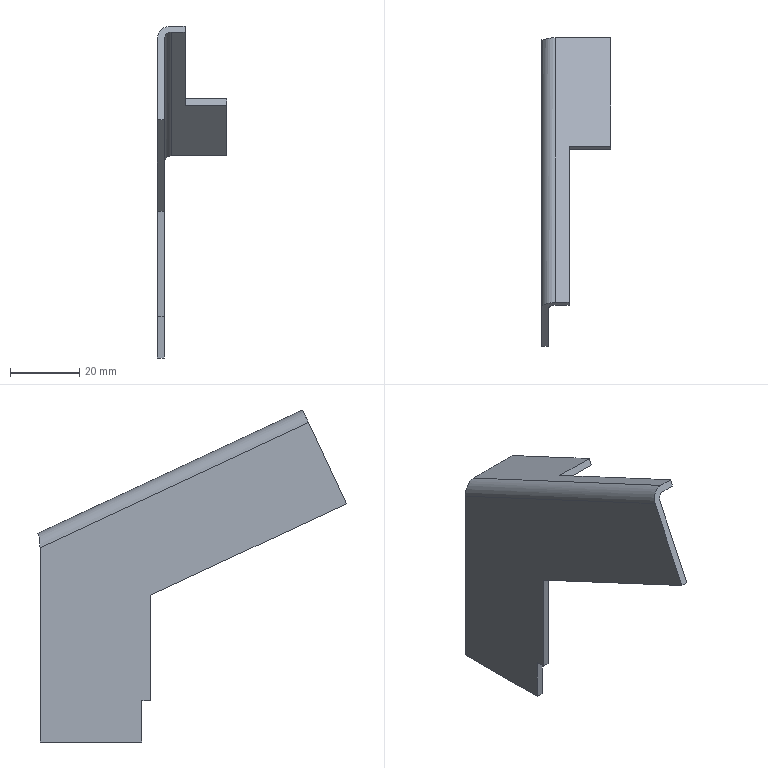Part | NX | features solid 2 | 1 solid | 18 faces | box 20 x 89.507 x 96.207 mm | volume 9278 mm3 | plane 15 | cylinder 2 | spline 1 | commonest cylinder face diameters 4 x1 8 x1
STEP:
#1=CARTESIAN_POINT('',(-260.,-1434.63,176.877));
#2=VERTEX_POINT('',#1);
#3=CARTESIAN_POINT('',(-272.,-1434.63,176.877));
#4=VERTEX_POINT('',#3);
#5=CARTESIAN_POINT('',(-280.,-1434.63,176.877));
#6=DIRECTION('',(-1.,0.,0.));
#7=VECTOR('',#6,1000.);
#8=LINE('',#5,#7);
#9=EDGE_CURVE('',#2,#4,#8,.T.);
#10=ORIENTED_EDGE('',*,*,#9,.F.);
#11=CARTESIAN_POINT('',(-260.,-1433.785,178.69));
#12=VERTEX_POINT('',#11);
#13=CARTESIAN_POINT('',(-260.,-1433.785,178.69));
#14=DIRECTION('',(0.,0.4226,0.9063));
#15=VECTOR('',#14,1000.);
#16=LINE('',#13,#15);
#17=EDGE_CURVE('',#2,#12,#16,.T.);
#18=ORIENTED_EDGE('',*,*,#17,.T.);
#19=CARTESIAN_POINT('',(-272.,-1433.785,178.69));
#20=VERTEX_POINT('',#19);
#21=CARTESIAN_POINT('',(-280.,-1433.785,178.69));
#22=DIRECTION('',(-1.,0.,0.));
#23=VECTOR('',#22,1000.);
#24=LINE('',#21,#23);
#25=EDGE_CURVE('',#12,#20,#24,.T.);
#26=ORIENTED_EDGE('',*,*,#25,.T.);
#27=CARTESIAN_POINT('',(-272.,-1433.785,178.69));
#28=DIRECTION('',(0.,0.4226,0.9063));
#29=VECTOR('',#28,1000.);
#30=LINE('',#27,#29);
#31=EDGE_CURVE('',#4,#20,#30,.T.);
#32=ORIENTED_EDGE('',*,*,#31,.F.);
#33=EDGE_LOOP('',(#10,#18,#26,#32));
#34=FACE_BOUND('',#33,.T.);
#35=CARTESIAN_POINT('',(-280.,-1433.785,178.69));
#36=DIRECTION('',(0.,0.9063,-0.4226));
#37=DIRECTION('',(-1.,0.,0.));
#38=AXIS2_PLACEMENT_3D('',#35,#36,#37);
#39=PLANE('',#38);
#40=ADVANCED_FACE('',(#34),#39,.F.);
#41=ORIENTED_EDGE('',*,*,#31,.T.);
#42=CARTESIAN_POINT('',(-272.,-1479.1,199.821));
#43=VERTEX_POINT('',#42);
#44=CARTESIAN_POINT('',(-272.,-1669.814,288.752));
#45=DIRECTION('',(0.,-0.9063,0.4226));
#46=VECTOR('',#45,1000.);
#47=LINE('',#44,#46);
#48=EDGE_CURVE('',#20,#43,#47,.T.);
#49=ORIENTED_EDGE('',*,*,#48,.T.);
#50=CARTESIAN_POINT('',(-272.,-1479.945,198.008));
#51=VERTEX_POINT('',#50);
#52=CARTESIAN_POINT('',(-272.,-1479.1,199.821));
#53=DIRECTION('',(0.,0.4226,0.9063));
#54=VECTOR('',#53,1000.);
#55=LINE('',#52,#54);
#56=EDGE_CURVE('',#51,#43,#55,.T.);
#57=ORIENTED_EDGE('',*,*,#56,.F.);
#58=CARTESIAN_POINT('',(-272.,-1670.659,286.939));
#59=DIRECTION('',(0.,-0.9063,0.4226));
#60=VECTOR('',#59,1000.);
#61=LINE('',#58,#60);
#62=EDGE_CURVE('',#4,#51,#61,.T.);
#63=ORIENTED_EDGE('',*,*,#62,.F.);
#64=EDGE_LOOP('',(#41,#49,#57,#63));
#65=FACE_BOUND('',#64,.T.);
#66=CARTESIAN_POINT('',(-272.,-1669.814,288.752));
#67=DIRECTION('',(-1.,0.,0.));
#68=DIRECTION('',(0.,0.,1.));
#69=AXIS2_PLACEMENT_3D('',#66,#67,#68);
#70=PLANE('',#69);
#71=ADVANCED_FACE('',(#65),#70,.F.);
#72=CARTESIAN_POINT('',(-278.,-1432.5,103.613));
#73=VERTEX_POINT('',#72);
#74=CARTESIAN_POINT('',(-278.,-1432.5,115.613));
#75=VERTEX_POINT('',#74);
#76=CARTESIAN_POINT('',(-278.,-1432.5,311.243));
#77=DIRECTION('',(0.,0.,1.));
#78=VECTOR('',#77,1000.);
#79=LINE('',#76,#78);
#80=EDGE_CURVE('',#73,#75,#79,.T.);
#81=ORIENTED_EDGE('',*,*,#80,.T.);
#82=CARTESIAN_POINT('',(-280.,-1432.5,115.613));
#83=VERTEX_POINT('',#82);
#84=CARTESIAN_POINT('',(-280.,-1432.5,115.613));
#85=DIRECTION('',(-1.,0.,0.));
#86=VECTOR('',#85,1000.);
#87=LINE('',#84,#86);
#88=EDGE_CURVE('',#75,#83,#87,.T.);
#89=ORIENTED_EDGE('',*,*,#88,.T.);
#90=CARTESIAN_POINT('',(-280.,-1432.5,103.613));
#91=VERTEX_POINT('',#90);
#92=CARTESIAN_POINT('',(-280.,-1432.5,311.243));
#93=DIRECTION('',(0.,0.,1.));
#94=VECTOR('',#93,1000.);
#95=LINE('',#92,#94);
#96=EDGE_CURVE('',#91,#83,#95,.T.);
#97=ORIENTED_EDGE('',*,*,#96,.F.);
#98=CARTESIAN_POINT('',(-280.,-1432.5,103.613));
#99=DIRECTION('',(-1.,0.,0.));
#100=VECTOR('',#99,1000.);
#101=LINE('',#98,#100);
#102=EDGE_CURVE('',#73,#91,#101,.T.);
#103=ORIENTED_EDGE('',*,*,#102,.F.);
#104=EDGE_LOOP('',(#81,#89,#97,#103));
#105=FACE_BOUND('',#104,.T.);
#106=CARTESIAN_POINT('',(-280.,-1432.5,311.243));
#107=DIRECTION('',(0.,1.,0.));
#108=DIRECTION('',(1.,0.,0.));
#109=AXIS2_PLACEMENT_3D('',#106,#107,#108);
#110=PLANE('',#109);
#111=ADVANCED_FACE('',(#105),#110,.F.);
#112=ORIENTED_EDGE('',*,*,#88,.F.);
#113=CARTESIAN_POINT('',(-278.,-1435.,115.613));
#114=VERTEX_POINT('',#113);
#115=CARTESIAN_POINT('',(-278.,-1650.,115.613));
#116=DIRECTION('',(0.,-1.,0.));
#117=VECTOR('',#116,1000.);
#118=LINE('',#115,#117);
#119=EDGE_CURVE('',#75,#114,#118,.T.);
#120=ORIENTED_EDGE('',*,*,#119,.T.);
#121=CARTESIAN_POINT('',(-280.,-1435.,115.613));
#122=VERTEX_POINT('',#121);
#123=CARTESIAN_POINT('',(-280.,-1435.,115.613));
#124=DIRECTION('',(-1.,0.,0.));
#125=VECTOR('',#124,1000.);
#126=LINE('',#123,#125);
#127=EDGE_CURVE('',#114,#122,#126,.T.);
#128=ORIENTED_EDGE('',*,*,#127,.T.);
#129=CARTESIAN_POINT('',(-280.,-1650.,115.613));
#130=DIRECTION('',(0.,-1.,0.));
#131=VECTOR('',#130,1000.);
#132=LINE('',#129,#131);
#133=EDGE_CURVE('',#83,#122,#132,.T.);
#134=ORIENTED_EDGE('',*,*,#133,.F.);
#135=EDGE_LOOP('',(#112,#120,#128,#134));
#136=FACE_BOUND('',#135,.T.);
#137=CARTESIAN_POINT('',(-280.,-1650.,115.613));
#138=DIRECTION('',(0.,0.,1.));
#139=DIRECTION('',(1.,0.,0.));
#140=AXIS2_PLACEMENT_3D('',#137,#138,#139);
#141=PLANE('',#140);
#142=ADVANCED_FACE('',(#136),#141,.F.);
#143=CARTESIAN_POINT('',(-278.,-1403.,159.921));
#144=VERTEX_POINT('',#143);
#145=CARTESIAN_POINT('',(-278.,-1480.791,196.195));
#146=VERTEX_POINT('',#145);
#147=CARTESIAN_POINT('',(-278.,-1403.,159.921));
#148=DIRECTION('',(0.,-0.9063,0.4226));
#149=VECTOR('',#148,1000.);
#150=LINE('',#147,#149);
#151=EDGE_CURVE('',#144,#146,#150,.T.);
#152=ORIENTED_EDGE('',*,*,#151,.F.);
#153=CARTESIAN_POINT('',(-277.414,-1403.365,161.652));
#154=VERTEX_POINT('',#153);
#155=CARTESIAN_POINT('',(-278.,-1403.,159.921));
#156=CARTESIAN_POINT('',(-278.,-1403.1,160.545));
#157=CARTESIAN_POINT('',(-277.784,-1403.201,161.166));
#158=CARTESIAN_POINT('',(-277.414,-1403.365,161.652));
#159=B_SPLINE_CURVE_WITH_KNOTS('',3,(#155,#156,#157,#158),.UNSPECIFIED.,.F.,.F.,(4,4),(0.,1.),.UNSPECIFIED.);
#160=EDGE_CURVE('',#154,#144,#159,.F.);
#161=ORIENTED_EDGE('',*,*,#160,.F.);
#162=CARTESIAN_POINT('',(-276.,-1403.117,162.182));
#163=VERTEX_POINT('',#162);
#164=CARTESIAN_POINT('',(-276.,-1403.963,160.37));
#165=DIRECTION('',(0.,0.9063,-0.4226));
#166=DIRECTION('',(-1.,0.,0.));
#167=AXIS2_PLACEMENT_3D('',#164,#165,#166);
#168=CIRCLE('',#167,2.);
#169=EDGE_CURVE('',#154,#163,#168,.T.);
#170=ORIENTED_EDGE('',*,*,#169,.T.);
#171=CARTESIAN_POINT('',(-276.,-1479.945,198.008));
#172=VERTEX_POINT('',#171);
#173=CARTESIAN_POINT('',(-276.,-1479.945,198.008));
#174=DIRECTION('',(0.,0.9063,-0.4226));
#175=VECTOR('',#174,1000.);
#176=LINE('',#173,#175);
#177=EDGE_CURVE('',#172,#163,#176,.T.);
#178=ORIENTED_EDGE('',*,*,#177,.F.);
#179=CARTESIAN_POINT('',(-276.,-1480.791,196.195));
#180=DIRECTION('',(0.,0.9063,-0.4226));
#181=DIRECTION('',(0.,0.4226,0.9063));
#182=AXIS2_PLACEMENT_3D('',#179,#180,#181);
#183=CIRCLE('',#182,2.);
#184=EDGE_CURVE('',#146,#172,#183,.T.);
#185=ORIENTED_EDGE('',*,*,#184,.F.);
#186=EDGE_LOOP('',(#152,#161,#170,#178,#185));
#187=FACE_BOUND('',#186,.T.);
#188=CARTESIAN_POINT('',(-276.,-1403.,159.921));
#189=DIRECTION('',(0.,-0.9063,0.4226));
#190=DIRECTION('',(1.,0.,0.));
#191=AXIS2_PLACEMENT_3D('',#188,#189,#190);
#192=CYLINDRICAL_SURFACE('',#191,2.);
#193=ADVANCED_FACE('',(#187),#192,.F.);
#194=CARTESIAN_POINT('',(-280.,-1403.,159.921));
#195=VERTEX_POINT('',#194);
#196=CARTESIAN_POINT('',(-280.,-1480.791,196.195));
#197=VERTEX_POINT('',#196);
#198=CARTESIAN_POINT('',(-280.,-1403.,159.921));
#199=DIRECTION('',(0.,-0.9063,0.4226));
#200=VECTOR('',#199,1000.);
#201=LINE('',#198,#200);
#202=EDGE_CURVE('',#195,#197,#201,.T.);
#203=ORIENTED_EDGE('',*,*,#202,.T.);
#204=CARTESIAN_POINT('',(-276.,-1479.1,199.821));
#205=VERTEX_POINT('',#204);
#206=CARTESIAN_POINT('',(-276.,-1480.791,196.195));
#207=DIRECTION('',(0.,0.9063,-0.4226));
#208=DIRECTION('',(1.,0.,0.));
#209=AXIS2_PLACEMENT_3D('',#206,#207,#208);
#210=CIRCLE('',#209,4.);
#211=EDGE_CURVE('',#197,#205,#210,.T.);
#212=ORIENTED_EDGE('',*,*,#211,.T.);
#213=CARTESIAN_POINT('',(-276.,-1402.272,163.995));
#214=VERTEX_POINT('',#213);
#215=CARTESIAN_POINT('',(-276.,-1479.1,199.821));
#216=DIRECTION('',(0.,0.9063,-0.4226));
#217=VECTOR('',#216,1000.);
#218=LINE('',#215,#217);
#219=EDGE_CURVE('',#205,#214,#218,.T.);
#220=ORIENTED_EDGE('',*,*,#219,.T.);
#221=CARTESIAN_POINT('',(-278.828,-1402.767,162.933));
#222=VERTEX_POINT('',#221);
#223=CARTESIAN_POINT('',(-276.,-1403.963,160.37));
#224=DIRECTION('',(0.,0.9063,-0.4226));
#225=DIRECTION('',(1.,0.,0.));
#226=AXIS2_PLACEMENT_3D('',#223,#224,#225);
#227=CIRCLE('',#226,4.);
#228=EDGE_CURVE('',#222,#214,#227,.T.);
#229=ORIENTED_EDGE('',*,*,#228,.F.);
#230=CARTESIAN_POINT('',(-278.828,-1402.767,162.933));
#231=CARTESIAN_POINT('',(-279.569,-1402.759,162.113));
#232=CARTESIAN_POINT('',(-280.,-1402.878,161.02));
#233=CARTESIAN_POINT('',(-280.,-1403.,159.921));
#234=B_SPLINE_CURVE_WITH_KNOTS('',3,(#230,#231,#232,#233),.UNSPECIFIED.,.F.,.F.,(4,4),(0.,1.),.UNSPECIFIED.);
#235=EDGE_CURVE('',#222,#195,#234,.T.);
#236=ORIENTED_EDGE('',*,*,#235,.T.);
#237=EDGE_LOOP('',(#203,#212,#220,#229,#236));
#238=FACE_BOUND('',#237,.T.);
#239=CARTESIAN_POINT('',(-276.,-1403.,159.921));
#240=DIRECTION('',(0.,-0.9063,0.4226));
#241=DIRECTION('',(1.,0.,0.));
#242=AXIS2_PLACEMENT_3D('',#239,#240,#241);
#243=CYLINDRICAL_SURFACE('',#242,4.);
#244=ADVANCED_FACE('',(#238),#243,.T.);
#245=ORIENTED_EDGE('',*,*,#160,.T.);
#246=CARTESIAN_POINT('',(-278.,-1403.,159.921));
#247=DIRECTION('',(-1.,0.,0.));
#248=VECTOR('',#247,1000.);
#249=LINE('',#246,#248);
#250=EDGE_CURVE('',#144,#195,#249,.T.);
#251=ORIENTED_EDGE('',*,*,#250,.T.);
#252=ORIENTED_EDGE('',*,*,#235,.F.);
#253=CARTESIAN_POINT('',(-278.828,-1402.767,162.933));
#254=DIRECTION('',(-0.7071,0.2988,0.6409));
#255=VECTOR('',#254,1000.);
#256=LINE('',#253,#255);
#257=EDGE_CURVE('',#154,#222,#256,.T.);
#258=ORIENTED_EDGE('',*,*,#257,.F.);
#259=EDGE_LOOP('',(#245,#251,#252,#258));
#260=FACE_BOUND('',#259,.T.);
#261=CARTESIAN_POINT('',(-278.828,-1402.767,162.933));
#262=CARTESIAN_POINT('',(-279.199,-1402.763,162.523));
#263=CARTESIAN_POINT('',(-279.495,-1402.79,162.046));
#264=CARTESIAN_POINT('',(-279.896,-1402.878,161.019));
#265=CARTESIAN_POINT('',(-280.,-1402.939,160.47));
#266=CARTESIAN_POINT('',(-280.,-1403.,159.921));
#267=CARTESIAN_POINT('',(-277.414,-1403.365,161.652));
#268=CARTESIAN_POINT('',(-277.599,-1403.283,161.409));
#269=CARTESIAN_POINT('',(-277.748,-1403.216,161.133));
#270=CARTESIAN_POINT('',(-277.948,-1403.1,160.545));
#271=CARTESIAN_POINT('',(-278.,-1403.05,160.233));
#272=CARTESIAN_POINT('',(-278.,-1403.,159.921));
#273=(BOUNDED_SURFACE()B_SPLINE_SURFACE(1,3,((#261,#262,#263,#264,#265,#266),(#267,#268,#269,#270,#271,#272)),.RULED_SURF.,.F.,.F.,.F.)B_SPLINE_SURFACE_WITH_KNOTS((2,2),(4,2,4),(0.,1.),(0.,0.5,1.),.UNSPECIFIED.)GEOMETRIC_REPRESENTATION_ITEM()RATIONAL_B_SPLINE_SURFACE(((1.,1.,1.,1.,1.,1.),(1.,1.,1.,1.,1.,1.)))REPRESENTATION_ITEM('')SURFACE());
#274=ADVANCED_FACE('',(#260),#273,.T.);
#275=ORIENTED_EDGE('',*,*,#9,.T.);
#276=ORIENTED_EDGE('',*,*,#62,.T.);
#277=CARTESIAN_POINT('',(-278.278,-1479.945,198.008));
#278=DIRECTION('',(-1.,0.,0.));
#279=VECTOR('',#278,1000.);
#280=LINE('',#277,#279);
#281=EDGE_CURVE('',#51,#172,#280,.T.);
#282=ORIENTED_EDGE('',*,*,#281,.T.);
#283=ORIENTED_EDGE('',*,*,#177,.T.);
#284=CARTESIAN_POINT('',(-260.,-1403.117,162.182));
#285=VERTEX_POINT('',#284);
#286=CARTESIAN_POINT('',(-278.278,-1403.117,162.182));
#287=DIRECTION('',(1.,0.,0.));
#288=VECTOR('',#287,1000.);
#289=LINE('',#286,#288);
#290=EDGE_CURVE('',#163,#285,#289,.T.);
#291=ORIENTED_EDGE('',*,*,#290,.T.);
#292=CARTESIAN_POINT('',(-260.,-1403.117,162.182));
#293=DIRECTION('',(0.,-0.9063,0.4226));
#294=VECTOR('',#293,1000.);
#295=LINE('',#292,#294);
#296=EDGE_CURVE('',#285,#2,#295,.T.);
#297=ORIENTED_EDGE('',*,*,#296,.T.);
#298=EDGE_LOOP('',(#275,#276,#282,#283,#291,#297));
#299=FACE_BOUND('',#298,.T.);
#300=CARTESIAN_POINT('',(-280.,-1670.659,286.939));
#301=DIRECTION('',(0.,0.4226,0.9063));
#302=DIRECTION('',(1.,0.,0.));
#303=AXIS2_PLACEMENT_3D('',#300,#301,#302);
#304=PLANE('',#303);
#305=ADVANCED_FACE('',(#299),#304,.F.);
#306=ORIENTED_EDGE('',*,*,#48,.F.);
#307=ORIENTED_EDGE('',*,*,#25,.F.);
#308=CARTESIAN_POINT('',(-260.,-1402.272,163.995));
#309=VERTEX_POINT('',#308);
#310=CARTESIAN_POINT('',(-260.,-1402.272,163.995));
#311=DIRECTION('',(0.,-0.9063,0.4226));
#312=VECTOR('',#311,1000.);
#313=LINE('',#310,#312);
#314=EDGE_CURVE('',#309,#12,#313,.T.);
#315=ORIENTED_EDGE('',*,*,#314,.F.);
#316=CARTESIAN_POINT('',(-278.278,-1402.272,163.995));
#317=DIRECTION('',(1.,0.,0.));
#318=VECTOR('',#317,1000.);
#319=LINE('',#316,#318);
#320=EDGE_CURVE('',#214,#309,#319,.T.);
#321=ORIENTED_EDGE('',*,*,#320,.F.);
#322=ORIENTED_EDGE('',*,*,#219,.F.);
#323=CARTESIAN_POINT('',(-278.278,-1479.1,199.821));
#324=DIRECTION('',(-1.,0.,0.));
#325=VECTOR('',#324,1000.);
#326=LINE('',#323,#325);
#327=EDGE_CURVE('',#43,#205,#326,.T.);
#328=ORIENTED_EDGE('',*,*,#327,.F.);
#329=EDGE_LOOP('',(#306,#307,#315,#321,#322,#328));
#330=FACE_BOUND('',#329,.T.);
#331=CARTESIAN_POINT('',(-280.,-1669.814,288.752));
#332=DIRECTION('',(0.,0.4226,0.9063));
#333=DIRECTION('',(1.,0.,0.));
#334=AXIS2_PLACEMENT_3D('',#331,#332,#333);
#335=PLANE('',#334);
#336=ADVANCED_FACE('',(#330),#335,.T.);
#337=ORIENTED_EDGE('',*,*,#320,.T.);
#338=CARTESIAN_POINT('',(-260.,-1402.272,163.995));
#339=DIRECTION('',(0.,-0.4226,-0.9063));
#340=VECTOR('',#339,1000.);
#341=LINE('',#338,#340);
#342=EDGE_CURVE('',#309,#285,#341,.T.);
#343=ORIENTED_EDGE('',*,*,#342,.T.);
#344=ORIENTED_EDGE('',*,*,#290,.F.);
#345=ORIENTED_EDGE('',*,*,#169,.F.);
#346=ORIENTED_EDGE('',*,*,#257,.T.);
#347=ORIENTED_EDGE('',*,*,#228,.T.);
#348=EDGE_LOOP('',(#337,#343,#344,#345,#346,#347));
#349=FACE_BOUND('',#348,.T.);
#350=CARTESIAN_POINT('',(-278.278,-1402.272,163.995));
#351=DIRECTION('',(0.,-0.9063,0.4226));
#352=DIRECTION('',(-1.,0.,0.));
#353=AXIS2_PLACEMENT_3D('',#350,#351,#352);
#354=PLANE('',#353);
#355=ADVANCED_FACE('',(#349),#354,.F.);
#356=ORIENTED_EDGE('',*,*,#80,.F.);
#357=CARTESIAN_POINT('',(-278.,-1403.,103.613));
#358=VERTEX_POINT('',#357);
#359=CARTESIAN_POINT('',(-278.,-1403.,103.613));
#360=DIRECTION('',(0.,-1.,0.));
#361=VECTOR('',#360,1000.);
#362=LINE('',#359,#361);
#363=EDGE_CURVE('',#358,#73,#362,.T.);
#364=ORIENTED_EDGE('',*,*,#363,.F.);
#365=CARTESIAN_POINT('',(-278.,-1403.,123.613));
#366=DIRECTION('',(0.,0.,-1.));
#367=VECTOR('',#366,1000.);
#368=LINE('',#365,#367);
#369=EDGE_CURVE('',#144,#358,#368,.T.);
#370=ORIENTED_EDGE('',*,*,#369,.F.);
#371=ORIENTED_EDGE('',*,*,#151,.T.);
#372=CARTESIAN_POINT('',(-278.,-1491.779,172.631));
#373=VERTEX_POINT('',#372);
#374=CARTESIAN_POINT('',(-278.,-1491.779,172.631));
#375=DIRECTION('',(0.,0.4226,0.9063));
#376=VECTOR('',#375,1000.);
#377=LINE('',#374,#376);
#378=EDGE_CURVE('',#373,#146,#377,.T.);
#379=ORIENTED_EDGE('',*,*,#378,.F.);
#380=CARTESIAN_POINT('',(-278.,-1435.,146.155));
#381=VERTEX_POINT('',#380);
#382=CARTESIAN_POINT('',(-278.,-1435.,146.155));
#383=DIRECTION('',(0.,-0.9063,0.4226));
#384=VECTOR('',#383,1000.);
#385=LINE('',#382,#384);
#386=EDGE_CURVE('',#381,#373,#385,.T.);
#387=ORIENTED_EDGE('',*,*,#386,.F.);
#388=CARTESIAN_POINT('',(-278.,-1435.,123.613));
#389=DIRECTION('',(0.,0.,1.));
#390=VECTOR('',#389,1000.);
#391=LINE('',#388,#390);
#392=EDGE_CURVE('',#114,#381,#391,.T.);
#393=ORIENTED_EDGE('',*,*,#392,.F.);
#394=ORIENTED_EDGE('',*,*,#119,.F.);
#395=EDGE_LOOP('',(#356,#364,#370,#371,#379,#387,#393,#394));
#396=FACE_BOUND('',#395,.T.);
#397=CARTESIAN_POINT('',(-278.,-1650.,331.243));
#398=DIRECTION('',(-1.,0.,0.));
#399=DIRECTION('',(0.,1.,0.));
#400=AXIS2_PLACEMENT_3D('',#397,#398,#399);
#401=PLANE('',#400);
#402=ADVANCED_FACE('',(#396),#401,.F.);
#403=CARTESIAN_POINT('',(-280.,-1435.,146.155));
#404=VERTEX_POINT('',#403);
#405=CARTESIAN_POINT('',(-280.,-1491.779,172.631));
#406=VERTEX_POINT('',#405);
#407=CARTESIAN_POINT('',(-280.,-1435.,146.155));
#408=DIRECTION('',(0.,-0.9063,0.4226));
#409=VECTOR('',#408,1000.);
#410=LINE('',#407,#409);
#411=EDGE_CURVE('',#404,#406,#410,.T.);
#412=ORIENTED_EDGE('',*,*,#411,.F.);
#413=CARTESIAN_POINT('',(-278.,-1435.,146.155));
#414=DIRECTION('',(-1.,0.,0.));
#415=VECTOR('',#414,1000.);
#416=LINE('',#413,#415);
#417=EDGE_CURVE('',#381,#404,#416,.T.);
#418=ORIENTED_EDGE('',*,*,#417,.F.);
#419=ORIENTED_EDGE('',*,*,#386,.T.);
#420=CARTESIAN_POINT('',(-278.,-1491.779,172.631));
#421=DIRECTION('',(-1.,0.,0.));
#422=VECTOR('',#421,1000.);
#423=LINE('',#420,#422);
#424=EDGE_CURVE('',#373,#406,#423,.T.);
#425=ORIENTED_EDGE('',*,*,#424,.T.);
#426=EDGE_LOOP('',(#412,#418,#419,#425));
#427=FACE_BOUND('',#426,.T.);
#428=CARTESIAN_POINT('',(-278.,-1435.,146.155));
#429=DIRECTION('',(0.,0.4226,0.9063));
#430=DIRECTION('',(1.,0.,0.));
#431=AXIS2_PLACEMENT_3D('',#428,#429,#430);
#432=PLANE('',#431);
#433=ADVANCED_FACE('',(#427),#432,.F.);
#434=ORIENTED_EDGE('',*,*,#392,.T.);
#435=ORIENTED_EDGE('',*,*,#417,.T.);
#436=CARTESIAN_POINT('',(-280.,-1435.,123.613));
#437=DIRECTION('',(0.,0.,1.));
#438=VECTOR('',#437,1000.);
#439=LINE('',#436,#438);
#440=EDGE_CURVE('',#122,#404,#439,.T.);
#441=ORIENTED_EDGE('',*,*,#440,.F.);
#442=ORIENTED_EDGE('',*,*,#127,.F.);
#443=EDGE_LOOP('',(#434,#435,#441,#442));
#444=FACE_BOUND('',#443,.T.);
#445=CARTESIAN_POINT('',(-278.,-1435.,123.613));
#446=DIRECTION('',(0.,1.,0.));
#447=DIRECTION('',(0.,0.,-1.));
#448=AXIS2_PLACEMENT_3D('',#445,#446,#447);
#449=PLANE('',#448);
#450=ADVANCED_FACE('',(#444),#449,.F.);
#451=ORIENTED_EDGE('',*,*,#133,.T.);
#452=ORIENTED_EDGE('',*,*,#440,.T.);
#453=ORIENTED_EDGE('',*,*,#411,.T.);
#454=CARTESIAN_POINT('',(-280.,-1491.779,172.631));
#455=DIRECTION('',(0.,0.4226,0.9063));
#456=VECTOR('',#455,1000.);
#457=LINE('',#454,#456);
#458=EDGE_CURVE('',#406,#197,#457,.T.);
#459=ORIENTED_EDGE('',*,*,#458,.T.);
#460=ORIENTED_EDGE('',*,*,#202,.F.);
#461=CARTESIAN_POINT('',(-280.,-1403.,103.613));
#462=VERTEX_POINT('',#461);
#463=CARTESIAN_POINT('',(-280.,-1403.,123.613));
#464=DIRECTION('',(0.,0.,-1.));
#465=VECTOR('',#464,1000.);
#466=LINE('',#463,#465);
#467=EDGE_CURVE('',#195,#462,#466,.T.);
#468=ORIENTED_EDGE('',*,*,#467,.T.);
#469=CARTESIAN_POINT('',(-280.,-1403.,103.613));
#470=DIRECTION('',(0.,-1.,0.));
#471=VECTOR('',#470,1000.);
#472=LINE('',#469,#471);
#473=EDGE_CURVE('',#462,#91,#472,.T.);
#474=ORIENTED_EDGE('',*,*,#473,.T.);
#475=ORIENTED_EDGE('',*,*,#96,.T.);
#476=EDGE_LOOP('',(#451,#452,#453,#459,#460,#468,#474,#475));
#477=FACE_BOUND('',#476,.T.);
#478=CARTESIAN_POINT('',(-280.,-1650.,331.243));
#479=DIRECTION('',(-1.,0.,0.));
#480=DIRECTION('',(0.,1.,0.));
#481=AXIS2_PLACEMENT_3D('',#478,#479,#480);
#482=PLANE('',#481);
#483=ADVANCED_FACE('',(#477),#482,.T.);
#484=ORIENTED_EDGE('',*,*,#369,.T.);
#485=CARTESIAN_POINT('',(-278.,-1403.,103.613));
#486=DIRECTION('',(-1.,0.,0.));
#487=VECTOR('',#486,1000.);
#488=LINE('',#485,#487);
#489=EDGE_CURVE('',#358,#462,#488,.T.);
#490=ORIENTED_EDGE('',*,*,#489,.T.);
#491=ORIENTED_EDGE('',*,*,#467,.F.);
#492=ORIENTED_EDGE('',*,*,#250,.F.);
#493=EDGE_LOOP('',(#484,#490,#491,#492));
#494=FACE_BOUND('',#493,.T.);
#495=CARTESIAN_POINT('',(-278.,-1403.,123.613));
#496=DIRECTION('',(0.,-1.,0.));
#497=DIRECTION('',(0.,0.,-1.));
#498=AXIS2_PLACEMENT_3D('',#495,#496,#497);
#499=PLANE('',#498);
#500=ADVANCED_FACE('',(#494),#499,.F.);
#501=ORIENTED_EDGE('',*,*,#281,.F.);
#502=ORIENTED_EDGE('',*,*,#56,.T.);
#503=ORIENTED_EDGE('',*,*,#327,.T.);
#504=ORIENTED_EDGE('',*,*,#211,.F.);
#505=ORIENTED_EDGE('',*,*,#458,.F.);
#506=ORIENTED_EDGE('',*,*,#424,.F.);
#507=ORIENTED_EDGE('',*,*,#378,.T.);
#508=ORIENTED_EDGE('',*,*,#184,.T.);
#509=EDGE_LOOP('',(#501,#502,#503,#504,#505,#506,#507,#508));
#510=FACE_BOUND('',#509,.T.);
#511=CARTESIAN_POINT('',(-278.,-1491.779,172.631));
#512=DIRECTION('',(0.,0.9063,-0.4226));
#513=DIRECTION('',(-1.,0.,0.));
#514=AXIS2_PLACEMENT_3D('',#511,#512,#513);
#515=PLANE('',#514);
#516=ADVANCED_FACE('',(#510),#515,.F.);
#517=ORIENTED_EDGE('',*,*,#102,.T.);
#518=ORIENTED_EDGE('',*,*,#473,.F.);
#519=ORIENTED_EDGE('',*,*,#489,.F.);
#520=ORIENTED_EDGE('',*,*,#363,.T.);
#521=EDGE_LOOP('',(#517,#518,#519,#520));
#522=FACE_BOUND('',#521,.T.);
#523=CARTESIAN_POINT('',(-278.,-1403.,103.613));
#524=DIRECTION('',(0.,0.,1.));
#525=DIRECTION('',(1.,0.,0.));
#526=AXIS2_PLACEMENT_3D('',#523,#524,#525);
#527=PLANE('',#526);
#528=ADVANCED_FACE('',(#522),#527,.F.);
#529=ORIENTED_EDGE('',*,*,#17,.F.);
#530=ORIENTED_EDGE('',*,*,#296,.F.);
#531=ORIENTED_EDGE('',*,*,#342,.F.);
#532=ORIENTED_EDGE('',*,*,#314,.T.);
#533=EDGE_LOOP('',(#529,#530,#531,#532));
#534=FACE_BOUND('',#533,.T.);
#535=CARTESIAN_POINT('',(-260.,-1402.272,163.995));
#536=DIRECTION('',(-1.,0.,0.));
#537=DIRECTION('',(0.,1.,0.));
#538=AXIS2_PLACEMENT_3D('',#535,#536,#537);
#539=PLANE('',#538);
#540=ADVANCED_FACE('',(#534),#539,.F.);
#541=CLOSED_SHELL('',(#40,#71,#111,#142,#193,#244,#274,#305,#336,#355,#402,#433,#450,#483,#500,#516,#528,#540));
#542=MANIFOLD_SOLID_BREP('',#541);
#543=(LENGTH_UNIT()NAMED_UNIT(*)SI_UNIT(.MILLI.,.METRE.));
#544=UNCERTAINTY_MEASURE_WITH_UNIT(LENGTH_MEASURE(0.0508),#543,'','');
#545=(NAMED_UNIT(*)PLANE_ANGLE_UNIT()SI_UNIT($,.RADIAN.));
#546=(NAMED_UNIT(*)SI_UNIT($,.STERADIAN.)SOLID_ANGLE_UNIT());
#547=(GEOMETRIC_REPRESENTATION_CONTEXT(3)GLOBAL_UNCERTAINTY_ASSIGNED_CONTEXT((#544))GLOBAL_UNIT_ASSIGNED_CONTEXT((#543,#545,#546))REPRESENTATION_CONTEXT('',''));
#548=ADVANCED_BREP_SHAPE_REPRESENTATION('',(#542),#547);